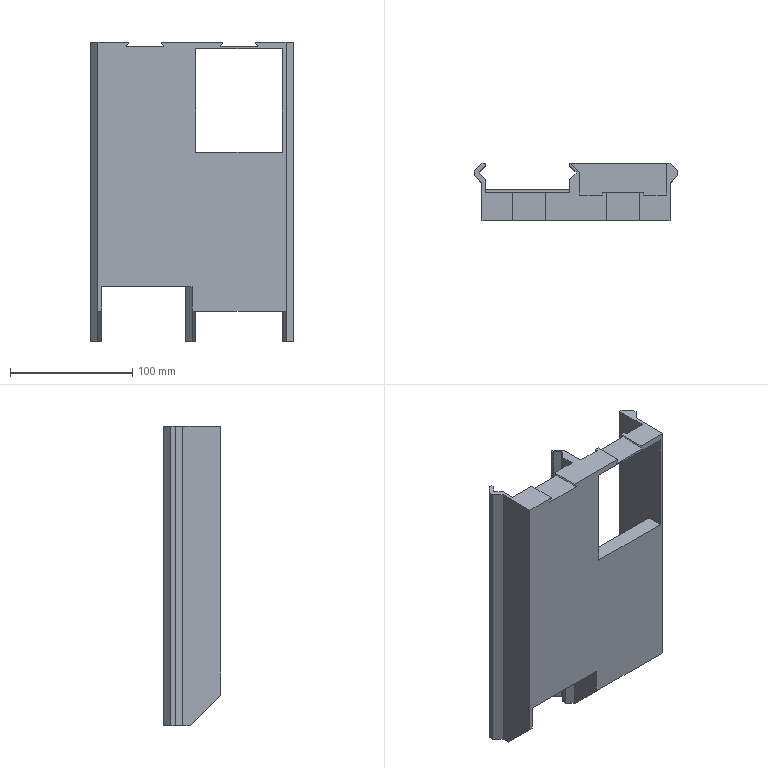Part | SolidWorks | features Cut 12, MoveFace 4, ICE 2, BossThin 1, Chamfer 1, CutThin 1, Extrusion 1 | 1 solid | 87 faces | box 166 x 47 x 245 mm | volume 294909 mm3 | plane 87